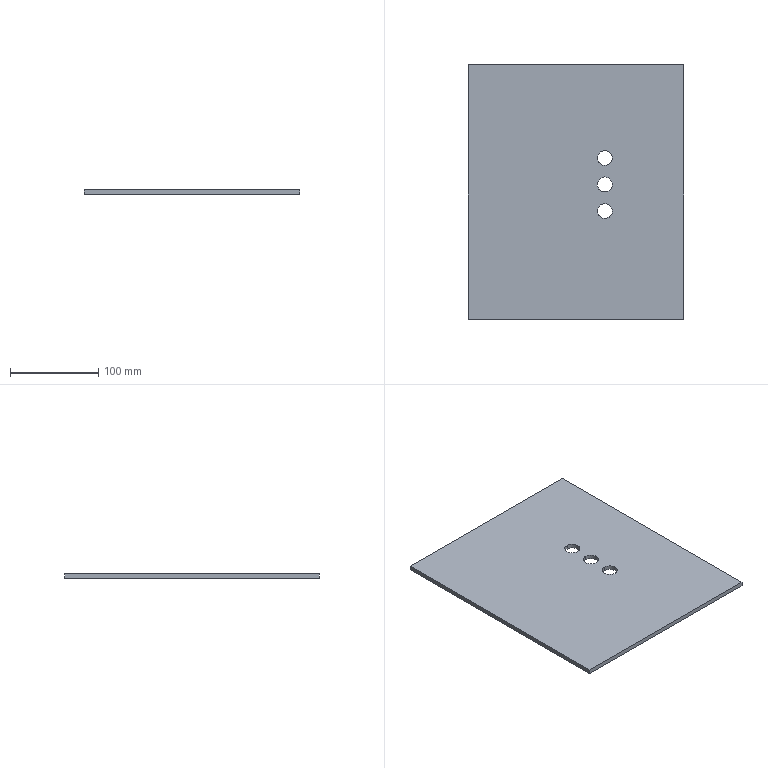Part | NX | features BREP 1 | 1 solid | 12 faces | box 243.37 x 288 x 5 mm | volume 347049 mm3 | cylinder 6 | plane 6 | commonest cylinder face diameters 17 x6
STEP:
#1=CARTESIAN_POINT('',(1894.999,-498.5,60.));
#2=VERTEX_POINT('',#1);
#3=CARTESIAN_POINT('',(1895.001,-481.5,60.));
#4=VERTEX_POINT('',#3);
#5=CARTESIAN_POINT('',(1895.,-498.5,60.));
#6=CARTESIAN_POINT('',(1895.974,-498.5,60.));
#7=CARTESIAN_POINT('',(1897.93,-498.172,60.));
#8=CARTESIAN_POINT('',(1901.646,-496.045,60.));
#9=CARTESIAN_POINT('',(1904.44,-490.737,60.));
#10=CARTESIAN_POINT('',(1902.023,-483.576,60.));
#11=CARTESIAN_POINT('',(1897.362,-481.5,60.));
#12=CARTESIAN_POINT('',(1895.001,-481.5,60.));
#13=B_SPLINE_CURVE_WITH_KNOTS('',3,(#5,#6,#7,#8,#9,#10,#11,#12),.UNSPECIFIED.,.F.,.F.,(4,1,1,1,1,4),(0.,0.125,0.25,0.5,0.75,1.),.UNSPECIFIED.);
#14=EDGE_CURVE('',#2,#4,#13,.T.);
#15=ORIENTED_EDGE('',*,*,#14,.F.);
#16=CARTESIAN_POINT('',(1895.001,-498.5,65.));
#17=VERTEX_POINT('',#16);
#18=CARTESIAN_POINT('',(1895.,-498.5,60.));
#19=CARTESIAN_POINT('',(1895.,-498.5,61.));
#20=CARTESIAN_POINT('',(1895.,-498.5,62.));
#21=CARTESIAN_POINT('',(1895.,-498.5,63.));
#22=CARTESIAN_POINT('',(1895.,-498.5,64.));
#23=CARTESIAN_POINT('',(1895.,-498.5,65.));
#24=(BOUNDED_CURVE()B_SPLINE_CURVE(5,(#18,#19,#20,#21,#22,#23),.UNSPECIFIED.,.F.,.F.)B_SPLINE_CURVE_WITH_KNOTS((6,6),(111.,116.),.UNSPECIFIED.)CURVE()GEOMETRIC_REPRESENTATION_ITEM()RATIONAL_B_SPLINE_CURVE((1.,1.,1.,1.,1.,1.))REPRESENTATION_ITEM(''));
#25=EDGE_CURVE('',#2,#17,#24,.T.);
#26=ORIENTED_EDGE('',*,*,#25,.T.);
#27=CARTESIAN_POINT('',(1894.999,-481.5,65.));
#28=VERTEX_POINT('',#27);
#29=CARTESIAN_POINT('',(1895.,-481.5,65.));
#30=CARTESIAN_POINT('',(1897.359,-481.5,65.));
#31=CARTESIAN_POINT('',(1902.023,-483.576,65.));
#32=CARTESIAN_POINT('',(1904.44,-490.736,65.));
#33=CARTESIAN_POINT('',(1901.647,-496.044,65.));
#34=CARTESIAN_POINT('',(1897.931,-498.171,65.));
#35=CARTESIAN_POINT('',(1895.976,-498.5,65.));
#36=CARTESIAN_POINT('',(1895.001,-498.5,65.));
#37=B_SPLINE_CURVE_WITH_KNOTS('',3,(#29,#30,#31,#32,#33,#34,#35,#36),.UNSPECIFIED.,.F.,.F.,(4,1,1,1,1,4),(0.,0.25,0.5,0.75,0.875,1.),.UNSPECIFIED.);
#38=EDGE_CURVE('',#17,#28,#37,.F.);
#39=ORIENTED_EDGE('',*,*,#38,.T.);
#40=CARTESIAN_POINT('',(1895.,-481.5,60.));
#41=CARTESIAN_POINT('',(1895.,-481.5,61.));
#42=CARTESIAN_POINT('',(1895.,-481.5,62.));
#43=CARTESIAN_POINT('',(1895.,-481.5,63.));
#44=CARTESIAN_POINT('',(1895.,-481.5,64.));
#45=CARTESIAN_POINT('',(1895.,-481.5,65.));
#46=(BOUNDED_CURVE()B_SPLINE_CURVE(5,(#40,#41,#42,#43,#44,#45),.UNSPECIFIED.,.F.,.F.)B_SPLINE_CURVE_WITH_KNOTS((6,6),(111.,116.),.UNSPECIFIED.)CURVE()GEOMETRIC_REPRESENTATION_ITEM()RATIONAL_B_SPLINE_CURVE((0.25,0.25,0.25,0.25,0.25,0.25))REPRESENTATION_ITEM(''));
#47=EDGE_CURVE('',#4,#28,#46,.T.);
#48=ORIENTED_EDGE('',*,*,#47,.F.);
#49=EDGE_LOOP('',(#15,#26,#39,#48));
#50=FACE_BOUND('',#49,.T.);
#51=CARTESIAN_POINT('',(1895.,-490.,49.));
#52=DIRECTION('',(0.,0.,1.));
#53=DIRECTION('',(0.,-1.,0.));
#54=AXIS2_PLACEMENT_3D('',#51,#52,#53);
#55=CYLINDRICAL_SURFACE('',#54,8.5);
#56=ADVANCED_FACE('',(#50),#55,.F.);
#57=CARTESIAN_POINT('',(1895.,-481.5,60.));
#58=CARTESIAN_POINT('',(1892.641,-481.5,60.));
#59=CARTESIAN_POINT('',(1887.977,-483.575,60.));
#60=CARTESIAN_POINT('',(1885.56,-490.735,60.));
#61=CARTESIAN_POINT('',(1888.352,-496.043,60.));
#62=CARTESIAN_POINT('',(1892.069,-498.171,60.));
#63=CARTESIAN_POINT('',(1894.024,-498.5,60.));
#64=CARTESIAN_POINT('',(1894.999,-498.5,60.));
#65=B_SPLINE_CURVE_WITH_KNOTS('',3,(#57,#58,#59,#60,#61,#62,#63,#64),.UNSPECIFIED.,.F.,.F.,(4,1,1,1,1,4),(0.,0.25,0.5,0.75,0.875,1.),.UNSPECIFIED.);
#66=EDGE_CURVE('',#4,#2,#65,.T.);
#67=ORIENTED_EDGE('',*,*,#66,.F.);
#68=ORIENTED_EDGE('',*,*,#47,.T.);
#69=CARTESIAN_POINT('',(1895.,-498.5,65.));
#70=CARTESIAN_POINT('',(1894.026,-498.5,65.));
#71=CARTESIAN_POINT('',(1892.069,-498.172,65.));
#72=CARTESIAN_POINT('',(1888.353,-496.044,65.));
#73=CARTESIAN_POINT('',(1885.56,-490.737,65.));
#74=CARTESIAN_POINT('',(1887.977,-483.576,65.));
#75=CARTESIAN_POINT('',(1892.639,-481.5,65.));
#76=CARTESIAN_POINT('',(1894.999,-481.5,65.));
#77=B_SPLINE_CURVE_WITH_KNOTS('',3,(#69,#70,#71,#72,#73,#74,#75,#76),.UNSPECIFIED.,.F.,.F.,(4,1,1,1,1,4),(0.,0.125,0.25,0.5,0.75,1.),.UNSPECIFIED.);
#78=EDGE_CURVE('',#28,#17,#77,.F.);
#79=ORIENTED_EDGE('',*,*,#78,.T.);
#80=ORIENTED_EDGE('',*,*,#25,.F.);
#81=EDGE_LOOP('',(#67,#68,#79,#80));
#82=FACE_BOUND('',#81,.T.);
#83=CARTESIAN_POINT('',(1895.,-490.,49.));
#84=DIRECTION('',(0.,0.,1.));
#85=DIRECTION('',(1.,0.,0.));
#86=AXIS2_PLACEMENT_3D('',#83,#84,#85);
#87=CYLINDRICAL_SURFACE('',#86,8.5);
#88=ADVANCED_FACE('',(#82),#87,.F.);
#89=CARTESIAN_POINT('',(1894.999,-468.5,60.));
#90=VERTEX_POINT('',#89);
#91=CARTESIAN_POINT('',(1895.001,-451.5,60.));
#92=VERTEX_POINT('',#91);
#93=CARTESIAN_POINT('',(1895.,-468.5,60.));
#94=CARTESIAN_POINT('',(1895.974,-468.5,60.));
#95=CARTESIAN_POINT('',(1897.93,-468.172,60.));
#96=CARTESIAN_POINT('',(1901.646,-466.045,60.));
#97=CARTESIAN_POINT('',(1904.44,-460.737,60.));
#98=CARTESIAN_POINT('',(1902.023,-453.576,60.));
#99=CARTESIAN_POINT('',(1897.362,-451.5,60.));
#100=CARTESIAN_POINT('',(1895.001,-451.5,60.));
#101=B_SPLINE_CURVE_WITH_KNOTS('',3,(#93,#94,#95,#96,#97,#98,#99,#100),.UNSPECIFIED.,.F.,.F.,(4,1,1,1,1,4),(0.,0.125,0.25,0.5,0.75,1.),.UNSPECIFIED.);
#102=EDGE_CURVE('',#90,#92,#101,.T.);
#103=ORIENTED_EDGE('',*,*,#102,.F.);
#104=CARTESIAN_POINT('',(1895.001,-468.5,65.));
#105=VERTEX_POINT('',#104);
#106=CARTESIAN_POINT('',(1895.,-468.5,60.));
#107=CARTESIAN_POINT('',(1895.,-468.5,61.));
#108=CARTESIAN_POINT('',(1895.,-468.5,62.));
#109=CARTESIAN_POINT('',(1895.,-468.5,63.));
#110=CARTESIAN_POINT('',(1895.,-468.5,64.));
#111=CARTESIAN_POINT('',(1895.,-468.5,65.));
#112=(BOUNDED_CURVE()B_SPLINE_CURVE(5,(#106,#107,#108,#109,#110,#111),.UNSPECIFIED.,.F.,.F.)B_SPLINE_CURVE_WITH_KNOTS((6,6),(111.,116.),.UNSPECIFIED.)CURVE()GEOMETRIC_REPRESENTATION_ITEM()RATIONAL_B_SPLINE_CURVE((1.,1.,1.,1.,1.,1.))REPRESENTATION_ITEM(''));
#113=EDGE_CURVE('',#90,#105,#112,.T.);
#114=ORIENTED_EDGE('',*,*,#113,.T.);
#115=CARTESIAN_POINT('',(1894.999,-451.5,65.));
#116=VERTEX_POINT('',#115);
#117=CARTESIAN_POINT('',(1895.,-451.5,65.));
#118=CARTESIAN_POINT('',(1897.359,-451.5,65.));
#119=CARTESIAN_POINT('',(1902.023,-453.576,65.));
#120=CARTESIAN_POINT('',(1904.44,-460.736,65.));
#121=CARTESIAN_POINT('',(1901.647,-466.044,65.));
#122=CARTESIAN_POINT('',(1897.931,-468.171,65.));
#123=CARTESIAN_POINT('',(1895.976,-468.5,65.));
#124=CARTESIAN_POINT('',(1895.001,-468.5,65.));
#125=B_SPLINE_CURVE_WITH_KNOTS('',3,(#117,#118,#119,#120,#121,#122,#123,#124),.UNSPECIFIED.,.F.,.F.,(4,1,1,1,1,4),(0.,0.25,0.5,0.75,0.875,1.),.UNSPECIFIED.);
#126=EDGE_CURVE('',#105,#116,#125,.F.);
#127=ORIENTED_EDGE('',*,*,#126,.T.);
#128=CARTESIAN_POINT('',(1895.,-451.5,60.));
#129=CARTESIAN_POINT('',(1895.,-451.5,61.));
#130=CARTESIAN_POINT('',(1895.,-451.5,62.));
#131=CARTESIAN_POINT('',(1895.,-451.5,63.));
#132=CARTESIAN_POINT('',(1895.,-451.5,64.));
#133=CARTESIAN_POINT('',(1895.,-451.5,65.));
#134=(BOUNDED_CURVE()B_SPLINE_CURVE(5,(#128,#129,#130,#131,#132,#133),.UNSPECIFIED.,.F.,.F.)B_SPLINE_CURVE_WITH_KNOTS((6,6),(111.,116.),.UNSPECIFIED.)CURVE()GEOMETRIC_REPRESENTATION_ITEM()RATIONAL_B_SPLINE_CURVE((0.25,0.25,0.25,0.25,0.25,0.25))REPRESENTATION_ITEM(''));
#135=EDGE_CURVE('',#92,#116,#134,.T.);
#136=ORIENTED_EDGE('',*,*,#135,.F.);
#137=EDGE_LOOP('',(#103,#114,#127,#136));
#138=FACE_BOUND('',#137,.T.);
#139=CARTESIAN_POINT('',(1895.,-460.,49.));
#140=DIRECTION('',(0.,0.,1.));
#141=DIRECTION('',(1.,0.,0.));
#142=AXIS2_PLACEMENT_3D('',#139,#140,#141);
#143=CYLINDRICAL_SURFACE('',#142,8.5);
#144=ADVANCED_FACE('',(#138),#143,.F.);
#145=CARTESIAN_POINT('',(1895.,-451.5,60.));
#146=CARTESIAN_POINT('',(1892.641,-451.5,60.));
#147=CARTESIAN_POINT('',(1887.977,-453.575,60.));
#148=CARTESIAN_POINT('',(1885.56,-460.735,60.));
#149=CARTESIAN_POINT('',(1888.352,-466.043,60.));
#150=CARTESIAN_POINT('',(1892.069,-468.171,60.));
#151=CARTESIAN_POINT('',(1894.024,-468.5,60.));
#152=CARTESIAN_POINT('',(1894.999,-468.5,60.));
#153=B_SPLINE_CURVE_WITH_KNOTS('',3,(#145,#146,#147,#148,#149,#150,#151,#152),.UNSPECIFIED.,.F.,.F.,(4,1,1,1,1,4),(0.,0.25,0.5,0.75,0.875,1.),.UNSPECIFIED.);
#154=EDGE_CURVE('',#92,#90,#153,.T.);
#155=ORIENTED_EDGE('',*,*,#154,.F.);
#156=ORIENTED_EDGE('',*,*,#135,.T.);
#157=CARTESIAN_POINT('',(1895.,-468.5,65.));
#158=CARTESIAN_POINT('',(1894.026,-468.5,65.));
#159=CARTESIAN_POINT('',(1892.069,-468.172,65.));
#160=CARTESIAN_POINT('',(1888.353,-466.044,65.));
#161=CARTESIAN_POINT('',(1885.56,-460.737,65.));
#162=CARTESIAN_POINT('',(1887.977,-453.576,65.));
#163=CARTESIAN_POINT('',(1892.639,-451.5,65.));
#164=CARTESIAN_POINT('',(1894.999,-451.5,65.));
#165=B_SPLINE_CURVE_WITH_KNOTS('',3,(#157,#158,#159,#160,#161,#162,#163,#164),.UNSPECIFIED.,.F.,.F.,(4,1,1,1,1,4),(0.,0.125,0.25,0.5,0.75,1.),.UNSPECIFIED.);
#166=EDGE_CURVE('',#116,#105,#165,.F.);
#167=ORIENTED_EDGE('',*,*,#166,.T.);
#168=ORIENTED_EDGE('',*,*,#113,.F.);
#169=EDGE_LOOP('',(#155,#156,#167,#168));
#170=FACE_BOUND('',#169,.T.);
#171=CARTESIAN_POINT('',(1895.,-460.,49.));
#172=DIRECTION('',(0.,0.,1.));
#173=DIRECTION('',(0.,-1.,0.));
#174=AXIS2_PLACEMENT_3D('',#171,#172,#173);
#175=CYLINDRICAL_SURFACE('',#174,8.5);
#176=ADVANCED_FACE('',(#170),#175,.F.);
#177=CARTESIAN_POINT('',(1894.999,-438.5,60.));
#178=VERTEX_POINT('',#177);
#179=CARTESIAN_POINT('',(1895.001,-421.5,60.));
#180=VERTEX_POINT('',#179);
#181=CARTESIAN_POINT('',(1895.,-438.5,60.));
#182=CARTESIAN_POINT('',(1895.974,-438.5,60.));
#183=CARTESIAN_POINT('',(1897.93,-438.172,60.));
#184=CARTESIAN_POINT('',(1901.646,-436.045,60.));
#185=CARTESIAN_POINT('',(1904.44,-430.737,60.));
#186=CARTESIAN_POINT('',(1902.023,-423.576,60.));
#187=CARTESIAN_POINT('',(1897.362,-421.5,60.));
#188=CARTESIAN_POINT('',(1895.001,-421.5,60.));
#189=B_SPLINE_CURVE_WITH_KNOTS('',3,(#181,#182,#183,#184,#185,#186,#187,#188),.UNSPECIFIED.,.F.,.F.,(4,1,1,1,1,4),(0.,0.125,0.25,0.5,0.75,1.),.UNSPECIFIED.);
#190=EDGE_CURVE('',#178,#180,#189,.T.);
#191=ORIENTED_EDGE('',*,*,#190,.F.);
#192=CARTESIAN_POINT('',(1895.,-438.5,65.));
#193=VERTEX_POINT('',#192);
#194=CARTESIAN_POINT('',(1895.,-438.5,60.));
#195=CARTESIAN_POINT('',(1895.,-438.5,61.));
#196=CARTESIAN_POINT('',(1895.,-438.5,62.));
#197=CARTESIAN_POINT('',(1895.,-438.5,63.));
#198=CARTESIAN_POINT('',(1895.,-438.5,64.));
#199=CARTESIAN_POINT('',(1895.,-438.5,65.));
#200=(BOUNDED_CURVE()B_SPLINE_CURVE(5,(#194,#195,#196,#197,#198,#199),.UNSPECIFIED.,.F.,.F.)B_SPLINE_CURVE_WITH_KNOTS((6,6),(111.,116.),.UNSPECIFIED.)CURVE()GEOMETRIC_REPRESENTATION_ITEM()RATIONAL_B_SPLINE_CURVE((1.,1.,1.,1.,1.,1.))REPRESENTATION_ITEM(''));
#201=EDGE_CURVE('',#178,#193,#200,.T.);
#202=ORIENTED_EDGE('',*,*,#201,.T.);
#203=CARTESIAN_POINT('',(1895.,-421.5,65.));
#204=VERTEX_POINT('',#203);
#205=CARTESIAN_POINT('',(1895.,-438.5,65.));
#206=CARTESIAN_POINT('',(1895.807,-438.5,65.));
#207=CARTESIAN_POINT('',(1896.636,-438.404,65.));
#208=CARTESIAN_POINT('',(1897.469,-438.202,65.));
#209=CARTESIAN_POINT('',(1899.048,-437.596,65.));
#210=CARTESIAN_POINT('',(1900.474,-436.585,65.));
#211=CARTESIAN_POINT('',(1901.109,-436.004,65.));
#212=CARTESIAN_POINT('',(1902.209,-434.702,65.));
#213=CARTESIAN_POINT('',(1902.968,-433.138,65.));
#214=CARTESIAN_POINT('',(1903.245,-432.321,65.));
#215=CARTESIAN_POINT('',(1903.584,-430.642,65.));
#216=CARTESIAN_POINT('',(1903.495,-428.91,65.));
#217=CARTESIAN_POINT('',(1903.343,-428.06,65.));
#218=CARTESIAN_POINT('',(1902.828,-426.42,65.));
#219=CARTESIAN_POINT('',(1901.916,-424.948,65.));
#220=CARTESIAN_POINT('',(1901.371,-424.276,65.));
#221=CARTESIAN_POINT('',(1900.125,-423.084,65.));
#222=CARTESIAN_POINT('',(1898.617,-422.236,65.));
#223=CARTESIAN_POINT('',(1897.815,-421.911,65.));
#224=CARTESIAN_POINT('',(1896.759,-421.631,65.));
#225=CARTESIAN_POINT('',(1895.679,-421.523,65.));
#226=CARTESIAN_POINT('',(1895.453,-421.508,65.));
#227=CARTESIAN_POINT('',(1895.227,-421.5,65.));
#228=CARTESIAN_POINT('',(1895.,-421.5,65.));
#229=B_SPLINE_CURVE_WITH_KNOTS('',5,(#205,#206,#207,#208,#209,#210,#211,#212,#213,#214,#215,#216,#217,#218,#219,#220,#221,#222,#223,#224,#225,#226,#227,#228),.UNSPECIFIED.,.F.,.F.,(6,3,3,3,3,3,3,6),(0.,6.667,12.918,18.932,24.809,30.609,36.373,37.896),.UNSPECIFIED.);
#230=EDGE_CURVE('',#193,#204,#229,.T.);
#231=ORIENTED_EDGE('',*,*,#230,.T.);
#232=CARTESIAN_POINT('',(1895.,-421.5,60.));
#233=CARTESIAN_POINT('',(1895.,-421.5,61.));
#234=CARTESIAN_POINT('',(1895.,-421.5,62.));
#235=CARTESIAN_POINT('',(1895.,-421.5,63.));
#236=CARTESIAN_POINT('',(1895.,-421.5,64.));
#237=CARTESIAN_POINT('',(1895.,-421.5,65.));
#238=(BOUNDED_CURVE()B_SPLINE_CURVE(5,(#232,#233,#234,#235,#236,#237),.UNSPECIFIED.,.F.,.F.)B_SPLINE_CURVE_WITH_KNOTS((6,6),(111.,116.),.UNSPECIFIED.)CURVE()GEOMETRIC_REPRESENTATION_ITEM()RATIONAL_B_SPLINE_CURVE((0.25,0.25,0.25,0.25,0.25,0.25))REPRESENTATION_ITEM(''));
#239=EDGE_CURVE('',#180,#204,#238,.T.);
#240=ORIENTED_EDGE('',*,*,#239,.F.);
#241=EDGE_LOOP('',(#191,#202,#231,#240));
#242=FACE_BOUND('',#241,.T.);
#243=CARTESIAN_POINT('',(1895.,-430.,49.));
#244=DIRECTION('',(0.,0.,1.));
#245=DIRECTION('',(1.,0.,0.));
#246=AXIS2_PLACEMENT_3D('',#243,#244,#245);
#247=CYLINDRICAL_SURFACE('',#246,8.5);
#248=ADVANCED_FACE('',(#242),#247,.F.);
#249=CARTESIAN_POINT('',(1895.,-421.5,60.));
#250=CARTESIAN_POINT('',(1892.641,-421.5,60.));
#251=CARTESIAN_POINT('',(1887.977,-423.575,60.));
#252=CARTESIAN_POINT('',(1885.56,-430.735,60.));
#253=CARTESIAN_POINT('',(1888.352,-436.043,60.));
#254=CARTESIAN_POINT('',(1892.069,-438.171,60.));
#255=CARTESIAN_POINT('',(1894.024,-438.5,60.));
#256=CARTESIAN_POINT('',(1894.999,-438.5,60.));
#257=B_SPLINE_CURVE_WITH_KNOTS('',3,(#249,#250,#251,#252,#253,#254,#255,#256),.UNSPECIFIED.,.F.,.F.,(4,1,1,1,1,4),(0.,0.25,0.5,0.75,0.875,1.),.UNSPECIFIED.);
#258=EDGE_CURVE('',#180,#178,#257,.T.);
#259=ORIENTED_EDGE('',*,*,#258,.F.);
#260=ORIENTED_EDGE('',*,*,#239,.T.);
#261=CARTESIAN_POINT('',(1895.,-438.5,65.));
#262=CARTESIAN_POINT('',(1894.024,-438.5,65.));
#263=CARTESIAN_POINT('',(1892.066,-438.171,65.));
#264=CARTESIAN_POINT('',(1888.348,-436.04,65.));
#265=CARTESIAN_POINT('',(1885.56,-430.728,65.));
#266=CARTESIAN_POINT('',(1887.982,-423.572,65.));
#267=CARTESIAN_POINT('',(1892.641,-421.5,65.));
#268=CARTESIAN_POINT('',(1895.,-421.5,65.));
#269=B_SPLINE_CURVE_WITH_KNOTS('',3,(#261,#262,#263,#264,#265,#266,#267,#268),.UNSPECIFIED.,.F.,.F.,(4,1,1,1,1,4),(0.,0.125,0.25,0.5,0.75,1.),.UNSPECIFIED.);
#270=EDGE_CURVE('',#204,#193,#269,.F.);
#271=ORIENTED_EDGE('',*,*,#270,.T.);
#272=ORIENTED_EDGE('',*,*,#201,.F.);
#273=EDGE_LOOP('',(#259,#260,#271,#272));
#274=FACE_BOUND('',#273,.T.);
#275=CARTESIAN_POINT('',(1895.,-430.,49.));
#276=DIRECTION('',(0.,0.,1.));
#277=DIRECTION('',(0.,-1.,0.));
#278=AXIS2_PLACEMENT_3D('',#275,#276,#277);
#279=CYLINDRICAL_SURFACE('',#278,8.5);
#280=ADVANCED_FACE('',(#274),#279,.F.);
#281=CARTESIAN_POINT('',(1740.711,-324.5,60.));
#282=VERTEX_POINT('',#281);
#283=CARTESIAN_POINT('',(1740.711,-324.5,65.));
#284=VERTEX_POINT('',#283);
#285=CARTESIAN_POINT('',(1740.711,-324.5,62.5));
#286=DIRECTION('',(0.,0.,1.));
#287=VECTOR('',#286,1000.);
#288=LINE('',#285,#287);
#289=EDGE_CURVE('',#282,#284,#288,.T.);
#290=ORIENTED_EDGE('',*,*,#289,.F.);
#291=CARTESIAN_POINT('',(1740.711,-612.5,60.));
#292=VERTEX_POINT('',#291);
#293=CARTESIAN_POINT('',(1740.711,-468.5,60.));
#294=DIRECTION('',(0.,1.,0.));
#295=VECTOR('',#294,1000.);
#296=LINE('',#293,#295);
#297=EDGE_CURVE('',#292,#282,#296,.T.);
#298=ORIENTED_EDGE('',*,*,#297,.F.);
#299=CARTESIAN_POINT('',(1740.711,-612.5,65.));
#300=VERTEX_POINT('',#299);
#301=CARTESIAN_POINT('',(1740.711,-612.5,62.5));
#302=DIRECTION('',(0.,0.,1.));
#303=VECTOR('',#302,1000.);
#304=LINE('',#301,#303);
#305=EDGE_CURVE('',#292,#300,#304,.T.);
#306=ORIENTED_EDGE('',*,*,#305,.T.);
#307=CARTESIAN_POINT('',(1740.711,-468.5,65.));
#308=DIRECTION('',(0.,1.,0.));
#309=VECTOR('',#308,1000.);
#310=LINE('',#307,#309);
#311=EDGE_CURVE('',#300,#284,#310,.T.);
#312=ORIENTED_EDGE('',*,*,#311,.T.);
#313=EDGE_LOOP('',(#290,#298,#306,#312));
#314=FACE_BOUND('',#313,.T.);
#315=CARTESIAN_POINT('',(1740.711,-468.5,65.));
#316=DIRECTION('',(1.,0.,0.));
#317=DIRECTION('',(0.,1.,0.));
#318=AXIS2_PLACEMENT_3D('',#315,#316,#317);
#319=PLANE('',#318);
#320=ADVANCED_FACE('',(#314),#319,.F.);
#321=ORIENTED_EDGE('',*,*,#38,.F.);
#322=ORIENTED_EDGE('',*,*,#78,.F.);
#323=EDGE_LOOP('',(#321,#322));
#324=FACE_BOUND('',#323,.T.);
#325=ORIENTED_EDGE('',*,*,#126,.F.);
#326=ORIENTED_EDGE('',*,*,#166,.F.);
#327=EDGE_LOOP('',(#325,#326));
#328=FACE_BOUND('',#327,.T.);
#329=ORIENTED_EDGE('',*,*,#230,.F.);
#330=ORIENTED_EDGE('',*,*,#270,.F.);
#331=EDGE_LOOP('',(#329,#330));
#332=FACE_BOUND('',#331,.T.);
#333=CARTESIAN_POINT('',(1984.081,-612.5,65.));
#334=VERTEX_POINT('',#333);
#335=CARTESIAN_POINT('',(1984.081,-324.5,65.));
#336=VERTEX_POINT('',#335);
#337=CARTESIAN_POINT('',(1984.081,-468.5,65.));
#338=DIRECTION('',(0.,1.,0.));
#339=VECTOR('',#338,1000.);
#340=LINE('',#337,#339);
#341=EDGE_CURVE('',#334,#336,#340,.T.);
#342=ORIENTED_EDGE('',*,*,#341,.T.);
#343=CARTESIAN_POINT('',(1862.396,-324.5,65.));
#344=DIRECTION('',(1.,0.,0.));
#345=VECTOR('',#344,1000.);
#346=LINE('',#343,#345);
#347=EDGE_CURVE('',#284,#336,#346,.T.);
#348=ORIENTED_EDGE('',*,*,#347,.F.);
#349=ORIENTED_EDGE('',*,*,#311,.F.);
#350=CARTESIAN_POINT('',(1862.396,-612.5,65.));
#351=DIRECTION('',(1.,0.,0.));
#352=VECTOR('',#351,1000.);
#353=LINE('',#350,#352);
#354=EDGE_CURVE('',#300,#334,#353,.T.);
#355=ORIENTED_EDGE('',*,*,#354,.T.);
#356=EDGE_LOOP('',(#342,#348,#349,#355));
#357=FACE_BOUND('',#356,.T.);
#358=CARTESIAN_POINT('',(0.,0.,65.));
#359=DIRECTION('',(0.,0.,-1.));
#360=DIRECTION('',(1.,0.,0.));
#361=AXIS2_PLACEMENT_3D('',#358,#359,#360);
#362=PLANE('',#361);
#363=ADVANCED_FACE('',(#324,#328,#332,#357),#362,.F.);
#364=CARTESIAN_POINT('',(1984.081,-324.5,60.));
#365=VERTEX_POINT('',#364);
#366=CARTESIAN_POINT('',(1984.081,-324.5,62.5));
#367=DIRECTION('',(0.,0.,-1.));
#368=VECTOR('',#367,1000.);
#369=LINE('',#366,#368);
#370=EDGE_CURVE('',#336,#365,#369,.T.);
#371=ORIENTED_EDGE('',*,*,#370,.T.);
#372=CARTESIAN_POINT('',(1862.396,-324.5,60.));
#373=DIRECTION('',(1.,0.,0.));
#374=VECTOR('',#373,1000.);
#375=LINE('',#372,#374);
#376=EDGE_CURVE('',#282,#365,#375,.T.);
#377=ORIENTED_EDGE('',*,*,#376,.F.);
#378=ORIENTED_EDGE('',*,*,#289,.T.);
#379=ORIENTED_EDGE('',*,*,#347,.T.);
#380=EDGE_LOOP('',(#371,#377,#378,#379));
#381=FACE_BOUND('',#380,.T.);
#382=CARTESIAN_POINT('',(1862.396,-324.5,65.));
#383=DIRECTION('',(0.,1.,0.));
#384=DIRECTION('',(1.,0.,0.));
#385=AXIS2_PLACEMENT_3D('',#382,#383,#384);
#386=PLANE('',#385);
#387=ADVANCED_FACE('',(#381),#386,.T.);
#388=ORIENTED_EDGE('',*,*,#66,.T.);
#389=ORIENTED_EDGE('',*,*,#14,.T.);
#390=EDGE_LOOP('',(#388,#389));
#391=FACE_BOUND('',#390,.T.);
#392=ORIENTED_EDGE('',*,*,#154,.T.);
#393=ORIENTED_EDGE('',*,*,#102,.T.);
#394=EDGE_LOOP('',(#392,#393));
#395=FACE_BOUND('',#394,.T.);
#396=ORIENTED_EDGE('',*,*,#258,.T.);
#397=ORIENTED_EDGE('',*,*,#190,.T.);
#398=EDGE_LOOP('',(#396,#397));
#399=FACE_BOUND('',#398,.T.);
#400=CARTESIAN_POINT('',(1984.081,-612.5,60.));
#401=VERTEX_POINT('',#400);
#402=CARTESIAN_POINT('',(1862.396,-612.5,60.));
#403=DIRECTION('',(1.,0.,0.));
#404=VECTOR('',#403,1000.);
#405=LINE('',#402,#404);
#406=EDGE_CURVE('',#292,#401,#405,.T.);
#407=ORIENTED_EDGE('',*,*,#406,.F.);
#408=ORIENTED_EDGE('',*,*,#297,.T.);
#409=ORIENTED_EDGE('',*,*,#376,.T.);
#410=CARTESIAN_POINT('',(1984.081,-468.5,60.));
#411=DIRECTION('',(0.,1.,0.));
#412=VECTOR('',#411,1000.);
#413=LINE('',#410,#412);
#414=EDGE_CURVE('',#401,#365,#413,.T.);
#415=ORIENTED_EDGE('',*,*,#414,.F.);
#416=EDGE_LOOP('',(#407,#408,#409,#415));
#417=FACE_BOUND('',#416,.T.);
#418=CARTESIAN_POINT('',(0.,0.,60.));
#419=DIRECTION('',(0.,0.,-1.));
#420=DIRECTION('',(1.,0.,0.));
#421=AXIS2_PLACEMENT_3D('',#418,#419,#420);
#422=PLANE('',#421);
#423=ADVANCED_FACE('',(#391,#395,#399,#417),#422,.T.);
#424=ORIENTED_EDGE('',*,*,#354,.F.);
#425=ORIENTED_EDGE('',*,*,#305,.F.);
#426=ORIENTED_EDGE('',*,*,#406,.T.);
#427=CARTESIAN_POINT('',(1984.081,-612.5,62.5));
#428=DIRECTION('',(0.,0.,-1.));
#429=VECTOR('',#428,1000.);
#430=LINE('',#427,#429);
#431=EDGE_CURVE('',#334,#401,#430,.T.);
#432=ORIENTED_EDGE('',*,*,#431,.F.);
#433=EDGE_LOOP('',(#424,#425,#426,#432));
#434=FACE_BOUND('',#433,.T.);
#435=CARTESIAN_POINT('',(1862.396,-612.5,65.));
#436=DIRECTION('',(0.,-1.,0.));
#437=DIRECTION('',(1.,0.,0.));
#438=AXIS2_PLACEMENT_3D('',#435,#436,#437);
#439=PLANE('',#438);
#440=ADVANCED_FACE('',(#434),#439,.T.);
#441=ORIENTED_EDGE('',*,*,#431,.T.);
#442=ORIENTED_EDGE('',*,*,#414,.T.);
#443=ORIENTED_EDGE('',*,*,#370,.F.);
#444=ORIENTED_EDGE('',*,*,#341,.F.);
#445=EDGE_LOOP('',(#441,#442,#443,#444));
#446=FACE_BOUND('',#445,.T.);
#447=CARTESIAN_POINT('',(1984.081,-468.5,65.));
#448=DIRECTION('',(-1.,0.,0.));
#449=DIRECTION('',(0.,1.,0.));
#450=AXIS2_PLACEMENT_3D('',#447,#448,#449);
#451=PLANE('',#450);
#452=ADVANCED_FACE('',(#446),#451,.F.);
#453=CLOSED_SHELL('',(#56,#88,#144,#176,#248,#280,#320,#363,#387,#423,#440,#452));
#454=MANIFOLD_SOLID_BREP('',#453);
#455=(LENGTH_UNIT()NAMED_UNIT(*)SI_UNIT(.MILLI.,.METRE.));
#456=UNCERTAINTY_MEASURE_WITH_UNIT(LENGTH_MEASURE(0.0508),#455,'','');
#457=(NAMED_UNIT(*)PLANE_ANGLE_UNIT()SI_UNIT($,.RADIAN.));
#458=(NAMED_UNIT(*)SI_UNIT($,.STERADIAN.)SOLID_ANGLE_UNIT());
#459=(GEOMETRIC_REPRESENTATION_CONTEXT(3)GLOBAL_UNCERTAINTY_ASSIGNED_CONTEXT((#456))GLOBAL_UNIT_ASSIGNED_CONTEXT((#455,#457,#458))REPRESENTATION_CONTEXT('',''));
#460=ADVANCED_BREP_SHAPE_REPRESENTATION('',(#454),#459);